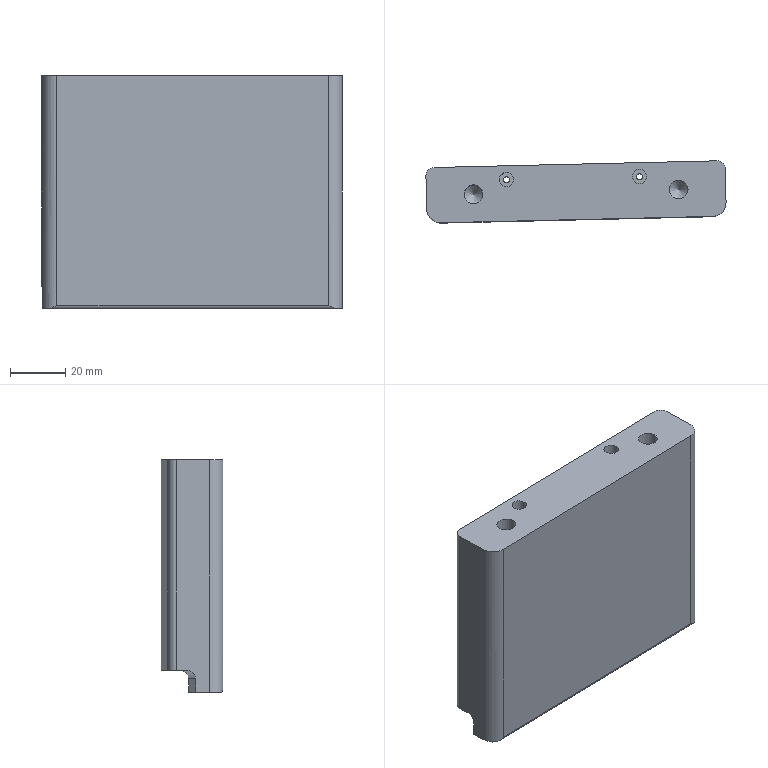Part | NX | features solid 2 | 1 solid | 26 faces | box 108.255 x 22.349 x 84 mm | volume 167370 mm3 | cylinder 13 | plane 10 | cone 3 | commonest cylinder face diameters 5.2 x3 6 x3 2.2 x2 6.8 x2 10 x2 2 x1
STEP:
#1=CARTESIAN_POINT('',(742.351,-102.251,-14.));
#2=VERTEX_POINT('',#1);
#3=CARTESIAN_POINT('',(740.446,-106.297,-14.));
#4=VERTEX_POINT('',#3);
#5=CARTESIAN_POINT('',(737.352,-102.368,-14.));
#6=DIRECTION('',(0.,0.,-1.));
#7=DIRECTION('',(-1.,0.,0.));
#8=AXIS2_PLACEMENT_3D('',#5,#6,#7);
#9=CIRCLE('',#8,5.);
#10=EDGE_CURVE('',#2,#4,#9,.T.);
#11=ORIENTED_EDGE('',*,*,#10,.T.);
#12=CARTESIAN_POINT('',(636.474,-108.743,-14.));
#13=VERTEX_POINT('',#12);
#14=CARTESIAN_POINT('',(16.573,-123.329,-14.));
#15=DIRECTION('',(-0.9997,-0.02352,0.));
#16=VECTOR('',#15,1000.);
#17=LINE('',#14,#16);
#18=EDGE_CURVE('',#4,#13,#17,.T.);
#19=ORIENTED_EDGE('',*,*,#18,.T.);
#20=CARTESIAN_POINT('',(634.381,-104.791,-14.));
#21=VERTEX_POINT('',#20);
#22=CARTESIAN_POINT('',(639.379,-104.674,-14.));
#23=DIRECTION('',(0.,0.,-1.));
#24=DIRECTION('',(-1.,0.,0.));
#25=AXIS2_PLACEMENT_3D('',#22,#23,#24);
#26=CIRCLE('',#25,5.);
#27=EDGE_CURVE('',#13,#21,#26,.T.);
#28=ORIENTED_EDGE('',*,*,#27,.T.);
#29=CARTESIAN_POINT('',(634.263,-99.793,-14.));
#30=VERTEX_POINT('',#29);
#31=CARTESIAN_POINT('',(634.028,-89.795,-14.));
#32=DIRECTION('',(0.02352,-0.9997,0.));
#33=VECTOR('',#32,1000.);
#34=LINE('',#31,#33);
#35=EDGE_CURVE('',#30,#21,#34,.T.);
#36=ORIENTED_EDGE('',*,*,#35,.F.);
#37=CARTESIAN_POINT('',(742.233,-97.252,-14.));
#38=VERTEX_POINT('',#37);
#39=CARTESIAN_POINT('',(688.248,-98.522,-14.));
#40=DIRECTION('',(0.9997,0.02352,0.));
#41=VECTOR('',#40,1000.);
#42=LINE('',#39,#41);
#43=EDGE_CURVE('',#30,#38,#42,.T.);
#44=ORIENTED_EDGE('',*,*,#43,.T.);
#45=CARTESIAN_POINT('',(742.084,-90.92,-14.));
#46=DIRECTION('',(-0.02352,0.9997,0.));
#47=VECTOR('',#46,1000.);
#48=LINE('',#45,#47);
#49=EDGE_CURVE('',#38,#2,#48,.F.);
#50=ORIENTED_EDGE('',*,*,#49,.T.);
#51=EDGE_LOOP('',(#11,#19,#28,#36,#44,#50));
#52=FACE_BOUND('',#51,.T.);
#53=CARTESIAN_POINT('',(685.766,-103.521,-14.));
#54=VERTEX_POINT('',#53);
#55=CARTESIAN_POINT('',(688.366,-103.521,-14.));
#56=DIRECTION('',(0.,0.,-1.));
#57=DIRECTION('',(-1.,0.,0.));
#58=AXIS2_PLACEMENT_3D('',#55,#56,#57);
#59=CIRCLE('',#58,2.6);
#60=EDGE_CURVE('',#54,#54,#59,.F.);
#61=ORIENTED_EDGE('',*,*,#60,.T.);
#62=EDGE_LOOP('',(#61));
#63=FACE_BOUND('',#62,.T.);
#64=CARTESIAN_POINT('',(16.212,-108.,-14.));
#65=DIRECTION('',(0.,0.,-1.));
#66=DIRECTION('',(-1.,0.,0.));
#67=AXIS2_PLACEMENT_3D('',#64,#65,#66);
#68=PLANE('',#67);
#69=ADVANCED_FACE('',(#52,#63),#68,.T.);
#70=CARTESIAN_POINT('',(728.638,-97.652,70.));
#71=VERTEX_POINT('',#70);
#72=CARTESIAN_POINT('',(725.238,-97.652,70.));
#73=DIRECTION('',(0.,0.,-1.));
#74=DIRECTION('',(1.,0.,0.));
#75=AXIS2_PLACEMENT_3D('',#72,#73,#74);
#76=CIRCLE('',#75,3.4);
#77=EDGE_CURVE('',#71,#71,#76,.T.);
#78=ORIENTED_EDGE('',*,*,#77,.T.);
#79=EDGE_LOOP('',(#78));
#80=FACE_BOUND('',#79,.T.);
#81=CARTESIAN_POINT('',(665.738,-94.112,70.));
#82=VERTEX_POINT('',#81);
#83=CARTESIAN_POINT('',(663.138,-94.112,70.));
#84=DIRECTION('',(0.,0.,1.));
#85=DIRECTION('',(1.,0.,0.));
#86=AXIS2_PLACEMENT_3D('',#83,#84,#85);
#87=CIRCLE('',#86,2.6);
#88=EDGE_CURVE('',#82,#82,#87,.T.);
#89=ORIENTED_EDGE('',*,*,#88,.F.);
#90=EDGE_LOOP('',(#89));
#91=FACE_BOUND('',#90,.T.);
#92=CARTESIAN_POINT('',(713.724,-92.983,70.));
#93=VERTEX_POINT('',#92);
#94=CARTESIAN_POINT('',(711.124,-92.983,70.));
#95=DIRECTION('',(0.,0.,1.));
#96=DIRECTION('',(1.,0.,0.));
#97=AXIS2_PLACEMENT_3D('',#94,#95,#96);
#98=CIRCLE('',#97,2.6);
#99=EDGE_CURVE('',#93,#93,#98,.T.);
#100=ORIENTED_EDGE('',*,*,#99,.F.);
#101=EDGE_LOOP('',(#100));
#102=FACE_BOUND('',#101,.T.);
#103=CARTESIAN_POINT('',(634.099,-92.795,70.));
#104=VERTEX_POINT('',#103);
#105=CARTESIAN_POINT('',(634.381,-104.791,70.));
#106=VERTEX_POINT('',#105);
#107=CARTESIAN_POINT('',(631.876,1.644,70.));
#108=DIRECTION('',(0.02352,-0.9997,0.));
#109=VECTOR('',#108,1000.);
#110=LINE('',#107,#109);
#111=EDGE_CURVE('',#104,#106,#110,.T.);
#112=ORIENTED_EDGE('',*,*,#111,.T.);
#113=CARTESIAN_POINT('',(639.497,-109.672,70.));
#114=VERTEX_POINT('',#113);
#115=CARTESIAN_POINT('',(639.379,-104.674,70.));
#116=DIRECTION('',(0.,0.,1.));
#117=DIRECTION('',(1.,0.,0.));
#118=AXIS2_PLACEMENT_3D('',#115,#116,#117);
#119=CIRCLE('',#118,5.);
#120=EDGE_CURVE('',#106,#114,#119,.T.);
#121=ORIENTED_EDGE('',*,*,#120,.T.);
#122=CARTESIAN_POINT('',(737.47,-107.367,70.));
#123=VERTEX_POINT('',#122);
#124=CARTESIAN_POINT('',(735.47,-107.414,70.));
#125=DIRECTION('',(-0.9997,-0.02352,0.));
#126=VECTOR('',#125,1000.);
#127=LINE('',#124,#126);
#128=EDGE_CURVE('',#123,#114,#127,.T.);
#129=ORIENTED_EDGE('',*,*,#128,.F.);
#130=CARTESIAN_POINT('',(742.351,-102.251,70.));
#131=VERTEX_POINT('',#130);
#132=CARTESIAN_POINT('',(737.352,-102.368,70.));
#133=DIRECTION('',(0.,0.,1.));
#134=DIRECTION('',(1.,0.,0.));
#135=AXIS2_PLACEMENT_3D('',#132,#133,#134);
#136=CIRCLE('',#135,5.);
#137=EDGE_CURVE('',#123,#131,#136,.T.);
#138=ORIENTED_EDGE('',*,*,#137,.T.);
#139=CARTESIAN_POINT('',(742.069,-90.254,70.));
#140=VERTEX_POINT('',#139);
#141=CARTESIAN_POINT('',(741.998,-87.255,70.));
#142=DIRECTION('',(-0.02352,0.9997,0.));
#143=VECTOR('',#142,1000.);
#144=LINE('',#141,#143);
#145=EDGE_CURVE('',#140,#131,#144,.F.);
#146=ORIENTED_EDGE('',*,*,#145,.F.);
#147=CARTESIAN_POINT('',(738.999,-87.325,70.));
#148=VERTEX_POINT('',#147);
#149=CARTESIAN_POINT('',(739.069,-90.325,70.));
#150=DIRECTION('',(0.,0.,1.));
#151=DIRECTION('',(1.,0.,0.));
#152=AXIS2_PLACEMENT_3D('',#149,#150,#151);
#153=CIRCLE('',#152,3.);
#154=EDGE_CURVE('',#140,#148,#153,.T.);
#155=ORIENTED_EDGE('',*,*,#154,.T.);
#156=CARTESIAN_POINT('',(637.027,-89.725,70.));
#157=VERTEX_POINT('',#156);
#158=CARTESIAN_POINT('',(735.,-87.419,70.));
#159=DIRECTION('',(-0.9997,-0.02352,0.));
#160=VECTOR('',#159,1000.);
#161=LINE('',#158,#160);
#162=EDGE_CURVE('',#148,#157,#161,.T.);
#163=ORIENTED_EDGE('',*,*,#162,.T.);
#164=CARTESIAN_POINT('',(637.098,-92.724,70.));
#165=DIRECTION('',(0.,0.,1.));
#166=DIRECTION('',(1.,0.,0.));
#167=AXIS2_PLACEMENT_3D('',#164,#165,#166);
#168=CIRCLE('',#167,3.);
#169=EDGE_CURVE('',#157,#104,#168,.T.);
#170=ORIENTED_EDGE('',*,*,#169,.T.);
#171=EDGE_LOOP('',(#112,#121,#129,#138,#146,#155,#163,#170));
#172=FACE_BOUND('',#171,.T.);
#173=CARTESIAN_POINT('',(654.658,-99.393,70.));
#174=VERTEX_POINT('',#173);
#175=CARTESIAN_POINT('',(651.258,-99.393,70.));
#176=DIRECTION('',(0.,0.,-1.));
#177=DIRECTION('',(1.,0.,0.));
#178=AXIS2_PLACEMENT_3D('',#175,#176,#177);
#179=CIRCLE('',#178,3.4);
#180=EDGE_CURVE('',#174,#174,#179,.T.);
#181=ORIENTED_EDGE('',*,*,#180,.T.);
#182=EDGE_LOOP('',(#181));
#183=FACE_BOUND('',#182,.T.);
#184=CARTESIAN_POINT('',(562.,0.,70.));
#185=DIRECTION('',(0.,0.,1.));
#186=DIRECTION('',(1.,0.,0.));
#187=AXIS2_PLACEMENT_3D('',#184,#185,#186);
#188=PLANE('',#187);
#189=ADVANCED_FACE('',(#80,#91,#102,#172,#183),#188,.T.);
#190=ORIENTED_EDGE('',*,*,#35,.T.);
#191=CARTESIAN_POINT('',(634.381,-104.791,50.));
#192=DIRECTION('',(0.,0.,-1.));
#193=VECTOR('',#192,1000.);
#194=LINE('',#191,#193);
#195=EDGE_CURVE('',#21,#106,#194,.F.);
#196=ORIENTED_EDGE('',*,*,#195,.T.);
#197=ORIENTED_EDGE('',*,*,#111,.F.);
#198=CARTESIAN_POINT('',(634.099,-92.795,-6.));
#199=VERTEX_POINT('',#198);
#200=CARTESIAN_POINT('',(634.099,-92.795,-58.));
#201=DIRECTION('',(0.,0.,-1.));
#202=VECTOR('',#201,1000.);
#203=LINE('',#200,#202);
#204=EDGE_CURVE('',#104,#199,#203,.T.);
#205=ORIENTED_EDGE('',*,*,#204,.T.);
#206=CARTESIAN_POINT('',(634.193,-96.793,-6.));
#207=VERTEX_POINT('',#206);
#208=CARTESIAN_POINT('',(634.028,-89.795,-6.));
#209=DIRECTION('',(-0.02352,0.9997,0.));
#210=VECTOR('',#209,1000.);
#211=LINE('',#208,#210);
#212=EDGE_CURVE('',#199,#207,#211,.F.);
#213=ORIENTED_EDGE('',*,*,#212,.T.);
#214=CARTESIAN_POINT('',(634.263,-99.793,-9.));
#215=VERTEX_POINT('',#214);
#216=CARTESIAN_POINT('',(634.193,-96.793,-9.));
#217=DIRECTION('',(-0.9997,-0.02352,0.));
#218=DIRECTION('',(0.02352,-0.9997,0.));
#219=AXIS2_PLACEMENT_3D('',#216,#217,#218);
#220=CIRCLE('',#219,3.);
#221=EDGE_CURVE('',#207,#215,#220,.F.);
#222=ORIENTED_EDGE('',*,*,#221,.T.);
#223=CARTESIAN_POINT('',(634.263,-99.793,50.));
#224=DIRECTION('',(0.,0.,1.));
#225=VECTOR('',#224,1000.);
#226=LINE('',#223,#225);
#227=EDGE_CURVE('',#30,#215,#226,.T.);
#228=ORIENTED_EDGE('',*,*,#227,.F.);
#229=EDGE_LOOP('',(#190,#196,#197,#205,#213,#222,#228));
#230=FACE_BOUND('',#229,.T.);
#231=CARTESIAN_POINT('',(634.028,-89.795,50.));
#232=DIRECTION('',(-0.9997,-0.02352,0.));
#233=DIRECTION('',(0.,0.,-1.));
#234=AXIS2_PLACEMENT_3D('',#231,#232,#233);
#235=PLANE('',#234);
#236=ADVANCED_FACE('',(#230),#235,.T.);
#237=CARTESIAN_POINT('',(664.238,-94.112,-6.));
#238=VERTEX_POINT('',#237);
#239=CARTESIAN_POINT('',(663.138,-94.112,-6.));
#240=DIRECTION('',(0.,0.,1.));
#241=DIRECTION('',(1.,0.,0.));
#242=AXIS2_PLACEMENT_3D('',#239,#240,#241);
#243=CIRCLE('',#242,1.1);
#244=EDGE_CURVE('',#238,#238,#243,.F.);
#245=ORIENTED_EDGE('',*,*,#244,.F.);
#246=EDGE_LOOP('',(#245));
#247=FACE_BOUND('',#246,.T.);
#248=CARTESIAN_POINT('',(712.224,-92.983,-6.));
#249=VERTEX_POINT('',#248);
#250=CARTESIAN_POINT('',(711.124,-92.983,-6.));
#251=DIRECTION('',(0.,0.,1.));
#252=DIRECTION('',(1.,0.,0.));
#253=AXIS2_PLACEMENT_3D('',#250,#251,#252);
#254=CIRCLE('',#253,1.1);
#255=EDGE_CURVE('',#249,#249,#254,.F.);
#256=ORIENTED_EDGE('',*,*,#255,.F.);
#257=EDGE_LOOP('',(#256));
#258=FACE_BOUND('',#257,.T.);
#259=CARTESIAN_POINT('',(742.069,-90.254,-6.));
#260=VERTEX_POINT('',#259);
#261=CARTESIAN_POINT('',(742.163,-94.253,-6.));
#262=VERTEX_POINT('',#261);
#263=CARTESIAN_POINT('',(741.998,-87.255,-6.));
#264=DIRECTION('',(0.02352,-0.9997,0.));
#265=VECTOR('',#264,1000.);
#266=LINE('',#263,#265);
#267=EDGE_CURVE('',#260,#262,#266,.T.);
#268=ORIENTED_EDGE('',*,*,#267,.T.);
#269=CARTESIAN_POINT('',(735.165,-94.418,-6.));
#270=DIRECTION('',(-0.9997,-0.02352,0.));
#271=VECTOR('',#270,1000.);
#272=LINE('',#269,#271);
#273=EDGE_CURVE('',#262,#207,#272,.T.);
#274=ORIENTED_EDGE('',*,*,#273,.T.);
#275=ORIENTED_EDGE('',*,*,#212,.F.);
#276=CARTESIAN_POINT('',(637.027,-89.725,-6.));
#277=VERTEX_POINT('',#276);
#278=CARTESIAN_POINT('',(637.098,-92.724,-6.));
#279=DIRECTION('',(0.,0.,1.));
#280=DIRECTION('',(1.,0.,0.));
#281=AXIS2_PLACEMENT_3D('',#278,#279,#280);
#282=CIRCLE('',#281,3.);
#283=EDGE_CURVE('',#199,#277,#282,.F.);
#284=ORIENTED_EDGE('',*,*,#283,.T.);
#285=CARTESIAN_POINT('',(738.999,-87.325,-6.));
#286=VERTEX_POINT('',#285);
#287=CARTESIAN_POINT('',(735.,-87.419,-6.));
#288=DIRECTION('',(0.9997,0.02352,0.));
#289=VECTOR('',#288,1000.);
#290=LINE('',#287,#289);
#291=EDGE_CURVE('',#286,#277,#290,.F.);
#292=ORIENTED_EDGE('',*,*,#291,.F.);
#293=CARTESIAN_POINT('',(739.069,-90.325,-6.));
#294=DIRECTION('',(0.,0.,1.));
#295=DIRECTION('',(1.,0.,0.));
#296=AXIS2_PLACEMENT_3D('',#293,#294,#295);
#297=CIRCLE('',#296,3.);
#298=EDGE_CURVE('',#286,#260,#297,.F.);
#299=ORIENTED_EDGE('',*,*,#298,.T.);
#300=EDGE_LOOP('',(#268,#274,#275,#284,#292,#299));
#301=FACE_BOUND('',#300,.T.);
#302=CARTESIAN_POINT('',(735.,-87.419,-6.));
#303=DIRECTION('',(0.,0.,1.));
#304=DIRECTION('',(-0.9997,-0.02352,0.));
#305=AXIS2_PLACEMENT_3D('',#302,#303,#304);
#306=PLANE('',#305);
#307=ADVANCED_FACE('',(#247,#258,#301),#306,.F.);
#308=ORIENTED_EDGE('',*,*,#145,.T.);
#309=CARTESIAN_POINT('',(742.351,-102.251,50.));
#310=DIRECTION('',(0.,0.,-1.));
#311=VECTOR('',#310,1000.);
#312=LINE('',#309,#311);
#313=EDGE_CURVE('',#131,#2,#312,.T.);
#314=ORIENTED_EDGE('',*,*,#313,.T.);
#315=ORIENTED_EDGE('',*,*,#49,.F.);
#316=CARTESIAN_POINT('',(742.233,-97.252,-9.));
#317=VERTEX_POINT('',#316);
#318=CARTESIAN_POINT('',(742.233,-97.252,50.));
#319=DIRECTION('',(0.,0.,1.));
#320=VECTOR('',#319,1000.);
#321=LINE('',#318,#320);
#322=EDGE_CURVE('',#317,#38,#321,.F.);
#323=ORIENTED_EDGE('',*,*,#322,.F.);
#324=CARTESIAN_POINT('',(742.163,-94.253,-9.));
#325=DIRECTION('',(-0.9997,-0.02352,0.));
#326=DIRECTION('',(0.02352,-0.9997,0.));
#327=AXIS2_PLACEMENT_3D('',#324,#325,#326);
#328=CIRCLE('',#327,3.);
#329=EDGE_CURVE('',#317,#262,#328,.T.);
#330=ORIENTED_EDGE('',*,*,#329,.T.);
#331=ORIENTED_EDGE('',*,*,#267,.F.);
#332=CARTESIAN_POINT('',(742.069,-90.254,50.));
#333=DIRECTION('',(0.,0.,-1.));
#334=VECTOR('',#333,1000.);
#335=LINE('',#332,#334);
#336=EDGE_CURVE('',#260,#140,#335,.F.);
#337=ORIENTED_EDGE('',*,*,#336,.T.);
#338=EDGE_LOOP('',(#308,#314,#315,#323,#330,#331,#337));
#339=FACE_BOUND('',#338,.T.);
#340=CARTESIAN_POINT('',(741.998,-87.255,50.));
#341=DIRECTION('',(-0.9997,-0.02352,0.));
#342=DIRECTION('',(0.,0.,-1.));
#343=AXIS2_PLACEMENT_3D('',#340,#341,#342);
#344=PLANE('',#343);
#345=ADVANCED_FACE('',(#339),#344,.F.);
#346=ORIENTED_EDGE('',*,*,#162,.F.);
#347=CARTESIAN_POINT('',(738.999,-87.325,-58.));
#348=DIRECTION('',(0.,0.,1.));
#349=VECTOR('',#348,1000.);
#350=LINE('',#347,#349);
#351=EDGE_CURVE('',#148,#286,#350,.F.);
#352=ORIENTED_EDGE('',*,*,#351,.T.);
#353=ORIENTED_EDGE('',*,*,#291,.T.);
#354=CARTESIAN_POINT('',(637.027,-89.725,50.));
#355=DIRECTION('',(0.,0.,-1.));
#356=VECTOR('',#355,1000.);
#357=LINE('',#354,#356);
#358=EDGE_CURVE('',#277,#157,#357,.F.);
#359=ORIENTED_EDGE('',*,*,#358,.T.);
#360=EDGE_LOOP('',(#346,#352,#353,#359));
#361=FACE_BOUND('',#360,.T.);
#362=CARTESIAN_POINT('',(735.,-87.419,50.));
#363=DIRECTION('',(0.02352,-0.9997,0.));
#364=DIRECTION('',(0.9997,0.02352,0.));
#365=AXIS2_PLACEMENT_3D('',#362,#363,#364);
#366=PLANE('',#365);
#367=ADVANCED_FACE('',(#361),#366,.F.);
#368=ORIENTED_EDGE('',*,*,#154,.F.);
#369=ORIENTED_EDGE('',*,*,#336,.F.);
#370=ORIENTED_EDGE('',*,*,#298,.F.);
#371=ORIENTED_EDGE('',*,*,#351,.F.);
#372=EDGE_LOOP('',(#368,#369,#370,#371));
#373=FACE_BOUND('',#372,.T.);
#374=CARTESIAN_POINT('',(739.069,-90.325,50.));
#375=DIRECTION('',(0.,0.,-1.));
#376=DIRECTION('',(-1.,0.,0.));
#377=AXIS2_PLACEMENT_3D('',#374,#375,#376);
#378=CYLINDRICAL_SURFACE('',#377,3.);
#379=ADVANCED_FACE('',(#373),#378,.T.);
#380=ORIENTED_EDGE('',*,*,#169,.F.);
#381=ORIENTED_EDGE('',*,*,#358,.F.);
#382=ORIENTED_EDGE('',*,*,#283,.F.);
#383=ORIENTED_EDGE('',*,*,#204,.F.);
#384=EDGE_LOOP('',(#380,#381,#382,#383));
#385=FACE_BOUND('',#384,.T.);
#386=CARTESIAN_POINT('',(637.098,-92.724,50.));
#387=DIRECTION('',(0.,0.,1.));
#388=DIRECTION('',(1.,0.,0.));
#389=AXIS2_PLACEMENT_3D('',#386,#387,#388);
#390=CYLINDRICAL_SURFACE('',#389,3.);
#391=ADVANCED_FACE('',(#385),#390,.T.);
#392=CARTESIAN_POINT('',(639.497,-109.672,-13.));
#393=VERTEX_POINT('',#392);
#394=CARTESIAN_POINT('',(639.497,-109.672,50.));
#395=DIRECTION('',(0.,0.,-1.));
#396=VECTOR('',#395,1000.);
#397=LINE('',#394,#396);
#398=EDGE_CURVE('',#114,#393,#397,.T.);
#399=ORIENTED_EDGE('',*,*,#398,.T.);
#400=CARTESIAN_POINT('',(737.47,-107.367,-13.));
#401=VERTEX_POINT('',#400);
#402=CARTESIAN_POINT('',(735.47,-107.414,-13.));
#403=DIRECTION('',(-0.9997,-0.02352,0.));
#404=VECTOR('',#403,1000.);
#405=LINE('',#402,#404);
#406=EDGE_CURVE('',#393,#401,#405,.F.);
#407=ORIENTED_EDGE('',*,*,#406,.T.);
#408=CARTESIAN_POINT('',(737.47,-107.367,50.));
#409=DIRECTION('',(0.,0.,1.));
#410=VECTOR('',#409,1000.);
#411=LINE('',#408,#410);
#412=EDGE_CURVE('',#401,#123,#411,.T.);
#413=ORIENTED_EDGE('',*,*,#412,.T.);
#414=ORIENTED_EDGE('',*,*,#128,.T.);
#415=EDGE_LOOP('',(#399,#407,#413,#414));
#416=FACE_BOUND('',#415,.T.);
#417=CARTESIAN_POINT('',(735.47,-107.414,50.));
#418=DIRECTION('',(0.02352,-0.9997,0.));
#419=DIRECTION('',(0.9997,0.02352,0.));
#420=AXIS2_PLACEMENT_3D('',#417,#418,#419);
#421=PLANE('',#420);
#422=ADVANCED_FACE('',(#416),#421,.T.);
#423=ORIENTED_EDGE('',*,*,#227,.T.);
#424=CARTESIAN_POINT('',(688.248,-98.522,-9.));
#425=DIRECTION('',(0.9997,0.02352,0.));
#426=VECTOR('',#425,1000.);
#427=LINE('',#424,#426);
#428=EDGE_CURVE('',#215,#317,#427,.T.);
#429=ORIENTED_EDGE('',*,*,#428,.T.);
#430=ORIENTED_EDGE('',*,*,#322,.T.);
#431=ORIENTED_EDGE('',*,*,#43,.F.);
#432=EDGE_LOOP('',(#423,#429,#430,#431));
#433=FACE_BOUND('',#432,.T.);
#434=CARTESIAN_POINT('',(688.248,-98.522,22.));
#435=DIRECTION('',(0.02352,-0.9997,0.));
#436=DIRECTION('',(0.9997,0.02352,0.));
#437=AXIS2_PLACEMENT_3D('',#434,#435,#436);
#438=PLANE('',#437);
#439=ADVANCED_FACE('',(#433),#438,.F.);
#440=ORIENTED_EDGE('',*,*,#329,.F.);
#441=ORIENTED_EDGE('',*,*,#428,.F.);
#442=ORIENTED_EDGE('',*,*,#221,.F.);
#443=ORIENTED_EDGE('',*,*,#273,.F.);
#444=EDGE_LOOP('',(#440,#441,#442,#443));
#445=FACE_BOUND('',#444,.T.);
#446=CARTESIAN_POINT('',(735.165,-94.418,-9.));
#447=DIRECTION('',(0.9997,0.02352,0.));
#448=DIRECTION('',(-0.02352,0.9997,0.));
#449=AXIS2_PLACEMENT_3D('',#446,#447,#448);
#450=CYLINDRICAL_SURFACE('',#449,3.);
#451=ADVANCED_FACE('',(#445),#450,.F.);
#452=ORIENTED_EDGE('',*,*,#27,.F.);
#453=CARTESIAN_POINT('',(636.474,-108.743,-14.));
#454=CARTESIAN_POINT('',(637.405,-109.408,-14.));
#455=CARTESIAN_POINT('',(638.467,-109.696,-13.461));
#456=CARTESIAN_POINT('',(639.497,-109.672,-13.));
#457=B_SPLINE_CURVE_WITH_KNOTS('',3,(#453,#454,#455,#456),.UNSPECIFIED.,.F.,.F.,(4,4),(0.,0.003386),.UNSPECIFIED.);
#458=EDGE_CURVE('',#13,#393,#457,.T.);
#459=ORIENTED_EDGE('',*,*,#458,.T.);
#460=ORIENTED_EDGE('',*,*,#398,.F.);
#461=ORIENTED_EDGE('',*,*,#120,.F.);
#462=ORIENTED_EDGE('',*,*,#195,.F.);
#463=EDGE_LOOP('',(#452,#459,#460,#461,#462));
#464=FACE_BOUND('',#463,.T.);
#465=CARTESIAN_POINT('',(639.379,-104.674,50.));
#466=DIRECTION('',(0.,0.,-1.));
#467=DIRECTION('',(-1.,0.,0.));
#468=AXIS2_PLACEMENT_3D('',#465,#466,#467);
#469=CYLINDRICAL_SURFACE('',#468,5.);
#470=ADVANCED_FACE('',(#464),#469,.T.);
#471=ORIENTED_EDGE('',*,*,#412,.F.);
#472=CARTESIAN_POINT('',(740.446,-106.297,-14.));
#473=CARTESIAN_POINT('',(739.547,-107.004,-14.));
#474=CARTESIAN_POINT('',(738.5,-107.343,-13.461));
#475=CARTESIAN_POINT('',(737.47,-107.367,-13.));
#476=B_SPLINE_CURVE_WITH_KNOTS('',3,(#472,#473,#474,#475),.UNSPECIFIED.,.F.,.F.,(4,4),(0.,0.003386),.UNSPECIFIED.);
#477=EDGE_CURVE('',#401,#4,#476,.F.);
#478=ORIENTED_EDGE('',*,*,#477,.T.);
#479=ORIENTED_EDGE('',*,*,#10,.F.);
#480=ORIENTED_EDGE('',*,*,#313,.F.);
#481=ORIENTED_EDGE('',*,*,#137,.F.);
#482=EDGE_LOOP('',(#471,#478,#479,#480,#481));
#483=FACE_BOUND('',#482,.T.);
#484=CARTESIAN_POINT('',(737.352,-102.368,50.));
#485=DIRECTION('',(0.,0.,1.));
#486=DIRECTION('',(1.,0.,0.));
#487=AXIS2_PLACEMENT_3D('',#484,#485,#486);
#488=CYLINDRICAL_SURFACE('',#487,5.);
#489=ADVANCED_FACE('',(#483),#488,.T.);
#490=ORIENTED_EDGE('',*,*,#477,.F.);
#491=ORIENTED_EDGE('',*,*,#406,.F.);
#492=ORIENTED_EDGE('',*,*,#458,.F.);
#493=ORIENTED_EDGE('',*,*,#18,.F.);
#494=EDGE_LOOP('',(#490,#491,#492,#493));
#495=FACE_BOUND('',#494,.T.);
#496=CARTESIAN_POINT('',(16.573,-123.329,-13.));
#497=DIRECTION('',(-0.9997,-0.02352,0.));
#498=DIRECTION('',(0.02352,-0.9997,0.));
#499=AXIS2_PLACEMENT_3D('',#496,#497,#498);
#500=CYLINDRICAL_SURFACE('',#499,1.);
#501=ADVANCED_FACE('',(#495),#500,.T.);
#502=ORIENTED_EDGE('',*,*,#255,.T.);
#503=EDGE_LOOP('',(#502));
#504=FACE_BOUND('',#503,.T.);
#505=CARTESIAN_POINT('',(710.024,-92.983,29.));
#506=VERTEX_POINT('',#505);
#507=CARTESIAN_POINT('',(711.124,-92.983,29.));
#508=DIRECTION('',(0.,0.,-1.));
#509=DIRECTION('',(-1.,0.,0.));
#510=AXIS2_PLACEMENT_3D('',#507,#508,#509);
#511=CIRCLE('',#510,1.1);
#512=EDGE_CURVE('',#506,#506,#511,.T.);
#513=ORIENTED_EDGE('',*,*,#512,.F.);
#514=EDGE_LOOP('',(#513));
#515=FACE_BOUND('',#514,.T.);
#516=CARTESIAN_POINT('',(711.124,-92.983,32.));
#517=DIRECTION('',(0.,0.,-1.));
#518=DIRECTION('',(1.,0.,0.));
#519=AXIS2_PLACEMENT_3D('',#516,#517,#518);
#520=CYLINDRICAL_SURFACE('',#519,1.1);
#521=ADVANCED_FACE('',(#504,#515),#520,.F.);
#522=ORIENTED_EDGE('',*,*,#512,.T.);
#523=EDGE_LOOP('',(#522));
#524=FACE_BOUND('',#523,.T.);
#525=CARTESIAN_POINT('',(713.724,-92.983,29.));
#526=VERTEX_POINT('',#525);
#527=CARTESIAN_POINT('',(711.124,-92.983,29.));
#528=DIRECTION('',(0.,0.,1.));
#529=DIRECTION('',(1.,0.,0.));
#530=AXIS2_PLACEMENT_3D('',#527,#528,#529);
#531=CIRCLE('',#530,2.6);
#532=EDGE_CURVE('',#526,#526,#531,.F.);
#533=ORIENTED_EDGE('',*,*,#532,.F.);
#534=EDGE_LOOP('',(#533));
#535=FACE_BOUND('',#534,.T.);
#536=CARTESIAN_POINT('',(711.124,-92.983,29.));
#537=DIRECTION('',(0.,0.,-1.));
#538=DIRECTION('',(-1.,0.,0.));
#539=AXIS2_PLACEMENT_3D('',#536,#537,#538);
#540=PLANE('',#539);
#541=ADVANCED_FACE('',(#524,#535),#540,.F.);
#542=ORIENTED_EDGE('',*,*,#99,.T.);
#543=EDGE_LOOP('',(#542));
#544=FACE_BOUND('',#543,.T.);
#545=ORIENTED_EDGE('',*,*,#532,.T.);
#546=EDGE_LOOP('',(#545));
#547=FACE_BOUND('',#546,.T.);
#548=CARTESIAN_POINT('',(711.124,-92.983,29.));
#549=DIRECTION('',(0.,0.,1.));
#550=DIRECTION('',(1.,0.,0.));
#551=AXIS2_PLACEMENT_3D('',#548,#549,#550);
#552=CYLINDRICAL_SURFACE('',#551,2.6);
#553=ADVANCED_FACE('',(#544,#547),#552,.F.);
#554=ORIENTED_EDGE('',*,*,#244,.T.);
#555=EDGE_LOOP('',(#554));
#556=FACE_BOUND('',#555,.T.);
#557=CARTESIAN_POINT('',(664.236,-94.06,29.));
#558=VERTEX_POINT('',#557);
#559=CARTESIAN_POINT('',(663.138,-94.112,29.));
#560=DIRECTION('',(0.,0.,1.));
#561=DIRECTION('',(0.9989,0.04703,0.));
#562=AXIS2_PLACEMENT_3D('',#559,#560,#561);
#563=CIRCLE('',#562,1.1);
#564=EDGE_CURVE('',#558,#558,#563,.T.);
#565=ORIENTED_EDGE('',*,*,#564,.T.);
#566=EDGE_LOOP('',(#565));
#567=FACE_BOUND('',#566,.T.);
#568=CARTESIAN_POINT('',(663.138,-94.112,32.));
#569=DIRECTION('',(0.,0.,-1.));
#570=DIRECTION('',(-0.9989,-0.04703,0.));
#571=AXIS2_PLACEMENT_3D('',#568,#569,#570);
#572=CYLINDRICAL_SURFACE('',#571,1.1);
#573=ADVANCED_FACE('',(#556,#567),#572,.F.);
#574=ORIENTED_EDGE('',*,*,#564,.F.);
#575=EDGE_LOOP('',(#574));
#576=FACE_BOUND('',#575,.T.);
#577=CARTESIAN_POINT('',(660.54,-94.234,29.));
#578=VERTEX_POINT('',#577);
#579=CARTESIAN_POINT('',(663.138,-94.112,29.));
#580=DIRECTION('',(0.,0.,-1.));
#581=DIRECTION('',(-0.9989,-0.04703,0.));
#582=AXIS2_PLACEMENT_3D('',#579,#580,#581);
#583=CIRCLE('',#582,2.6);
#584=EDGE_CURVE('',#578,#578,#583,.F.);
#585=ORIENTED_EDGE('',*,*,#584,.T.);
#586=EDGE_LOOP('',(#585));
#587=FACE_BOUND('',#586,.T.);
#588=CARTESIAN_POINT('',(663.138,-94.112,29.));
#589=DIRECTION('',(0.,0.,-1.));
#590=DIRECTION('',(0.9989,0.04703,0.));
#591=AXIS2_PLACEMENT_3D('',#588,#589,#590);
#592=PLANE('',#591);
#593=ADVANCED_FACE('',(#576,#587),#592,.F.);
#594=ORIENTED_EDGE('',*,*,#88,.T.);
#595=EDGE_LOOP('',(#594));
#596=FACE_BOUND('',#595,.T.);
#597=ORIENTED_EDGE('',*,*,#584,.F.);
#598=EDGE_LOOP('',(#597));
#599=FACE_BOUND('',#598,.T.);
#600=CARTESIAN_POINT('',(663.138,-94.112,29.));
#601=DIRECTION('',(0.,0.,1.));
#602=DIRECTION('',(-0.9989,-0.04703,0.));
#603=AXIS2_PLACEMENT_3D('',#600,#601,#602);
#604=CYLINDRICAL_SURFACE('',#603,2.6);
#605=ADVANCED_FACE('',(#596,#599),#604,.F.);
#606=CARTESIAN_POINT('',(721.838,-97.652,44.4));
#607=VERTEX_POINT('',#606);
#608=CARTESIAN_POINT('',(725.238,-97.652,44.4));
#609=DIRECTION('',(0.,0.,-1.));
#610=DIRECTION('',(-1.,0.,0.));
#611=AXIS2_PLACEMENT_3D('',#608,#609,#610);
#612=CIRCLE('',#611,3.4);
#613=EDGE_CURVE('',#607,#607,#612,.T.);
#614=ORIENTED_EDGE('',*,*,#613,.T.);
#615=EDGE_LOOP('',(#614));
#616=FACE_BOUND('',#615,.T.);
#617=ORIENTED_EDGE('',*,*,#77,.F.);
#618=EDGE_LOOP('',(#617));
#619=FACE_BOUND('',#618,.T.);
#620=CARTESIAN_POINT('',(725.238,-97.652,70.));
#621=DIRECTION('',(0.,0.,-1.));
#622=DIRECTION('',(1.,0.,0.));
#623=AXIS2_PLACEMENT_3D('',#620,#621,#622);
#624=CYLINDRICAL_SURFACE('',#623,3.4);
#625=ADVANCED_FACE('',(#616,#619),#624,.F.);
#626=CARTESIAN_POINT('',(725.238,-97.652,41.));
#627=VERTEX_POINT('',#626);
#628=VERTEX_LOOP('',#627);
#629=FACE_BOUND('',#628,.T.);
#630=ORIENTED_EDGE('',*,*,#613,.F.);
#631=EDGE_LOOP('',(#630));
#632=FACE_BOUND('',#631,.T.);
#633=CARTESIAN_POINT('',(725.238,-97.652,44.4));
#634=DIRECTION('',(0.,0.,1.));
#635=DIRECTION('',(1.,0.,0.));
#636=AXIS2_PLACEMENT_3D('',#633,#634,#635);
#637=CONICAL_SURFACE('',#636,3.4,0.7854);
#638=ADVANCED_FACE('',(#629,#632),#637,.F.);
#639=CARTESIAN_POINT('',(647.858,-99.393,44.4));
#640=VERTEX_POINT('',#639);
#641=CARTESIAN_POINT('',(651.258,-99.393,44.4));
#642=DIRECTION('',(0.,0.,-1.));
#643=DIRECTION('',(-1.,0.,0.));
#644=AXIS2_PLACEMENT_3D('',#641,#642,#643);
#645=CIRCLE('',#644,3.4);
#646=EDGE_CURVE('',#640,#640,#645,.T.);
#647=ORIENTED_EDGE('',*,*,#646,.T.);
#648=EDGE_LOOP('',(#647));
#649=FACE_BOUND('',#648,.T.);
#650=ORIENTED_EDGE('',*,*,#180,.F.);
#651=EDGE_LOOP('',(#650));
#652=FACE_BOUND('',#651,.T.);
#653=CARTESIAN_POINT('',(651.258,-99.393,70.));
#654=DIRECTION('',(0.,0.,-1.));
#655=DIRECTION('',(1.,0.,0.));
#656=AXIS2_PLACEMENT_3D('',#653,#654,#655);
#657=CYLINDRICAL_SURFACE('',#656,3.4);
#658=ADVANCED_FACE('',(#649,#652),#657,.F.);
#659=CARTESIAN_POINT('',(651.258,-99.393,41.));
#660=VERTEX_POINT('',#659);
#661=VERTEX_LOOP('',#660);
#662=FACE_BOUND('',#661,.T.);
#663=ORIENTED_EDGE('',*,*,#646,.F.);
#664=EDGE_LOOP('',(#663));
#665=FACE_BOUND('',#664,.T.);
#666=CARTESIAN_POINT('',(651.258,-99.393,44.4));
#667=DIRECTION('',(0.,0.,1.));
#668=DIRECTION('',(1.,0.,0.));
#669=AXIS2_PLACEMENT_3D('',#666,#667,#668);
#670=CONICAL_SURFACE('',#669,3.4,0.7854);
#671=ADVANCED_FACE('',(#662,#665),#670,.F.);
#672=CARTESIAN_POINT('',(685.766,-103.521,7.4));
#673=VERTEX_POINT('',#672);
#674=CARTESIAN_POINT('',(688.366,-103.521,7.4));
#675=DIRECTION('',(0.,0.,-1.));
#676=DIRECTION('',(-1.,0.,0.));
#677=AXIS2_PLACEMENT_3D('',#674,#675,#676);
#678=CIRCLE('',#677,2.6);
#679=EDGE_CURVE('',#673,#673,#678,.F.);
#680=ORIENTED_EDGE('',*,*,#679,.T.);
#681=EDGE_LOOP('',(#680));
#682=FACE_BOUND('',#681,.T.);
#683=ORIENTED_EDGE('',*,*,#60,.F.);
#684=EDGE_LOOP('',(#683));
#685=FACE_BOUND('',#684,.T.);
#686=CARTESIAN_POINT('',(688.366,-103.521,-14.));
#687=DIRECTION('',(0.,0.,1.));
#688=DIRECTION('',(1.,0.,0.));
#689=AXIS2_PLACEMENT_3D('',#686,#687,#688);
#690=CYLINDRICAL_SURFACE('',#689,2.6);
#691=ADVANCED_FACE('',(#682,#685),#690,.F.);
#692=CARTESIAN_POINT('',(688.366,-103.521,10.));
#693=VERTEX_POINT('',#692);
#694=VERTEX_LOOP('',#693);
#695=FACE_BOUND('',#694,.T.);
#696=ORIENTED_EDGE('',*,*,#679,.F.);
#697=EDGE_LOOP('',(#696));
#698=FACE_BOUND('',#697,.T.);
#699=CARTESIAN_POINT('',(688.366,-103.521,7.401));
#700=DIRECTION('',(0.,0.,-1.));
#701=DIRECTION('',(-1.,0.,0.));
#702=AXIS2_PLACEMENT_3D('',#699,#700,#701);
#703=CONICAL_SURFACE('',#702,2.599,0.7854);
#704=ADVANCED_FACE('',(#695,#698),#703,.F.);
#705=CLOSED_SHELL('',(#69,#189,#236,#307,#345,#367,#379,#391,#422,#439,#451,#470,#489,#501,#521,#541,#553,#573,#593,#605,#625,#638,#658,#671,#691,#704));
#706=MANIFOLD_SOLID_BREP('',#705);
#707=(LENGTH_UNIT()NAMED_UNIT(*)SI_UNIT(.MILLI.,.METRE.));
#708=UNCERTAINTY_MEASURE_WITH_UNIT(LENGTH_MEASURE(0.0508),#707,'','');
#709=(NAMED_UNIT(*)PLANE_ANGLE_UNIT()SI_UNIT($,.RADIAN.));
#710=(NAMED_UNIT(*)SI_UNIT($,.STERADIAN.)SOLID_ANGLE_UNIT());
#711=(GEOMETRIC_REPRESENTATION_CONTEXT(3)GLOBAL_UNCERTAINTY_ASSIGNED_CONTEXT((#708))GLOBAL_UNIT_ASSIGNED_CONTEXT((#707,#709,#710))REPRESENTATION_CONTEXT('',''));
#712=ADVANCED_BREP_SHAPE_REPRESENTATION('',(#706),#711);